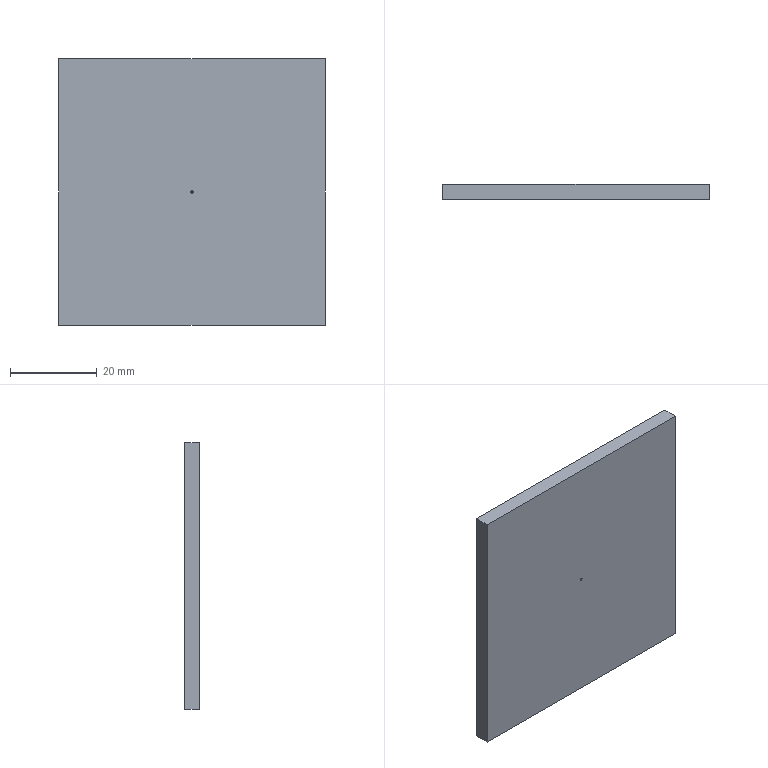Part | STEP file | 1 solid | 8 faces | box 61.25 x 3.43 x 61.25 mm | volume 12867 mm3 | plane 6 | cylinder 2 | commonest cylinder face diameters 0.49 x2
STEP:
#1=CARTESIAN_POINT('',(0.,0.,0.));
#2=DIRECTION('',(0.,0.,1.));
#3=DIRECTION('',(1.,0.,0.));
#4=AXIS2_PLACEMENT_3D('',#1,#2,#3);
#5=CARTESIAN_POINT('',(949.794,-61.739,161.762));
#6=VERTEX_POINT('',#5);
#7=CARTESIAN_POINT('',(950.284,-61.739,161.762));
#8=VERTEX_POINT('',#7);
#9=CARTESIAN_POINT('',(950.039,-61.739,161.762));
#10=DIRECTION('',(0.,-1.,0.));
#11=DIRECTION('',(-1.,0.,0.));
#12=AXIS2_PLACEMENT_3D('',#9,#10,#11);
#13=CIRCLE('',#12,0.245);
#14=CARTESIAN_POINT('',(950.039,-56.839,161.762));
#15=DIRECTION('',(0.,-1.,0.));
#16=DIRECTION('',(-1.,0.,0.));
#17=AXIS2_PLACEMENT_3D('',#14,#15,#16);
#18=CYLINDRICAL_SURFACE('',#17,0.245);
#19=CARTESIAN_POINT('',(0.,4.9));
#20=DIRECTION('',(1.,0.));
#21=VECTOR('',#20,1.);
#22=LINE('',#19,#21);
#23=(GEOMETRIC_REPRESENTATION_CONTEXT(2)PARAMETRIC_REPRESENTATION_CONTEXT()REPRESENTATION_CONTEXT('',''));
#24=DEFINITIONAL_REPRESENTATION('',(#22),#23);
#25=PCURVE('',#18,#24);
#26=CARTESIAN_POINT('',(980.664,-61.739,131.137));
#27=DIRECTION('',(0.,1.,0.));
#28=DIRECTION('',(0.,0.,-1.));
#29=AXIS2_PLACEMENT_3D('',#26,#27,#28);
#30=PLANE('',#29);
#31=CARTESIAN_POINT('',(-30.625,30.87));
#32=CARTESIAN_POINT('',(-30.201,30.87));
#33=CARTESIAN_POINT('',(-30.413,30.503));
#34=CARTESIAN_POINT('',(-30.625,30.135));
#35=CARTESIAN_POINT('',(-30.837,30.503));
#36=CARTESIAN_POINT('',(-31.049,30.87));
#37=CARTESIAN_POINT('',(-30.625,30.87));
#38=(BOUNDED_CURVE()B_SPLINE_CURVE(2,(#31,#32,#33,#34,#35,#36,#37),.UNSPECIFIED.,.T.,.F.)B_SPLINE_CURVE_WITH_KNOTS((1,2,2,2,2,1),(-2.094,0.,2.094,4.189,6.283,8.378),.UNSPECIFIED.)CURVE()GEOMETRIC_REPRESENTATION_ITEM()RATIONAL_B_SPLINE_CURVE((1.,0.5,1.,0.5,1.,0.5,1.))REPRESENTATION_ITEM(''));
#39=(GEOMETRIC_REPRESENTATION_CONTEXT(2)PARAMETRIC_REPRESENTATION_CONTEXT()REPRESENTATION_CONTEXT('',''));
#40=DEFINITIONAL_REPRESENTATION('',(#38),#39);
#41=PCURVE('',#30,#40);
#42=SURFACE_CURVE('',#13,(#25,#41),.PCURVE_S1.);
#43=EDGE_CURVE('',#6,#8,#42,.T.);
#44=ORIENTED_EDGE('',*,*,#43,.F.);
#45=CARTESIAN_POINT('',(949.794,-58.309,161.762));
#46=VERTEX_POINT('',#45);
#47=CARTESIAN_POINT('',(949.794,-56.839,161.762));
#48=DIRECTION('',(0.,-1.,0.));
#49=VECTOR('',#48,1.);
#50=LINE('',#47,#49);
#51=CARTESIAN_POINT('',(0.,0.));
#52=DIRECTION('',(0.,1.));
#53=VECTOR('',#52,1.);
#54=LINE('',#51,#53);
#55=(GEOMETRIC_REPRESENTATION_CONTEXT(2)PARAMETRIC_REPRESENTATION_CONTEXT()REPRESENTATION_CONTEXT('',''));
#56=DEFINITIONAL_REPRESENTATION('',(#54),#55);
#57=PCURVE('',#18,#56);
#58=CARTESIAN_POINT('',(950.039,-56.839,161.762));
#59=DIRECTION('',(0.,-1.,0.));
#60=DIRECTION('',(-1.,0.,0.));
#61=AXIS2_PLACEMENT_3D('',#58,#59,#60);
#62=CYLINDRICAL_SURFACE('',#61,0.245);
#63=CARTESIAN_POINT('',(6.283,0.));
#64=DIRECTION('',(0.,1.));
#65=VECTOR('',#64,1.);
#66=LINE('',#63,#65);
#67=(GEOMETRIC_REPRESENTATION_CONTEXT(2)PARAMETRIC_REPRESENTATION_CONTEXT()REPRESENTATION_CONTEXT('',''));
#68=DEFINITIONAL_REPRESENTATION('',(#66),#67);
#69=PCURVE('',#62,#68);
#70=SURFACE_CURVE('',#50,(#57,#69),.PCURVE_S1.);
#71=EDGE_CURVE('',#46,#6,#70,.T.);
#72=ORIENTED_EDGE('',*,*,#71,.F.);
#73=CARTESIAN_POINT('',(950.284,-58.309,161.762));
#74=VERTEX_POINT('',#73);
#75=CARTESIAN_POINT('',(950.039,-58.309,161.762));
#76=DIRECTION('',(0.,1.,0.));
#77=DIRECTION('',(1.,0.,0.));
#78=AXIS2_PLACEMENT_3D('',#75,#76,#77);
#79=CIRCLE('',#78,0.245);
#80=CARTESIAN_POINT('',(3.142,1.47));
#81=DIRECTION('',(-1.,0.));
#82=VECTOR('',#81,1.);
#83=LINE('',#80,#82);
#84=(GEOMETRIC_REPRESENTATION_CONTEXT(2)PARAMETRIC_REPRESENTATION_CONTEXT()REPRESENTATION_CONTEXT('',''));
#85=DEFINITIONAL_REPRESENTATION('',(#83),#84);
#86=PCURVE('',#18,#85);
#87=CARTESIAN_POINT('',(980.664,-58.309,131.137));
#88=DIRECTION('',(0.,1.,0.));
#89=DIRECTION('',(0.,0.,-1.));
#90=AXIS2_PLACEMENT_3D('',#87,#88,#89);
#91=PLANE('',#90);
#92=CARTESIAN_POINT('',(-30.625,30.625));
#93=DIRECTION('',(0.,-1.));
#94=AXIS2_PLACEMENT_2D('',#92,#93);
#95=CIRCLE('',#94,0.245);
#96=(GEOMETRIC_REPRESENTATION_CONTEXT(2)PARAMETRIC_REPRESENTATION_CONTEXT()REPRESENTATION_CONTEXT('',''));
#97=DEFINITIONAL_REPRESENTATION('',(#95),#96);
#98=PCURVE('',#91,#97);
#99=SURFACE_CURVE('',#79,(#86,#98),.PCURVE_S1.);
#100=EDGE_CURVE('',#74,#46,#99,.T.);
#101=ORIENTED_EDGE('',*,*,#100,.F.);
#102=CARTESIAN_POINT('',(950.284,-56.839,161.762));
#103=DIRECTION('',(0.,-1.,0.));
#104=VECTOR('',#103,1.);
#105=LINE('',#102,#104);
#106=CARTESIAN_POINT('',(3.142,0.));
#107=DIRECTION('',(0.,1.));
#108=VECTOR('',#107,1.);
#109=LINE('',#106,#108);
#110=(GEOMETRIC_REPRESENTATION_CONTEXT(2)PARAMETRIC_REPRESENTATION_CONTEXT()REPRESENTATION_CONTEXT('',''));
#111=DEFINITIONAL_REPRESENTATION('',(#109),#110);
#112=PCURVE('',#18,#111);
#113=CARTESIAN_POINT('',(3.142,0.));
#114=DIRECTION('',(0.,1.));
#115=VECTOR('',#114,1.);
#116=LINE('',#113,#115);
#117=(GEOMETRIC_REPRESENTATION_CONTEXT(2)PARAMETRIC_REPRESENTATION_CONTEXT()REPRESENTATION_CONTEXT('',''));
#118=DEFINITIONAL_REPRESENTATION('',(#116),#117);
#119=PCURVE('',#62,#118);
#120=SURFACE_CURVE('',#105,(#112,#119),.PCURVE_S1.);
#121=EDGE_CURVE('',#74,#8,#120,.T.);
#122=ORIENTED_EDGE('',*,*,#121,.T.);
#123=EDGE_LOOP('',(#44,#72,#101,#122));
#124=FACE_BOUND('',#123,.F.);
#125=ADVANCED_FACE('',(#124),#18,.F.);
#126=CARTESIAN_POINT('',(980.664,-61.739,192.387));
#127=VERTEX_POINT('',#126);
#128=CARTESIAN_POINT('',(919.414,-61.739,192.387));
#129=VERTEX_POINT('',#128);
#130=CARTESIAN_POINT('',(980.664,-61.739,192.387));
#131=DIRECTION('',(-1.,0.,0.));
#132=VECTOR('',#131,1.);
#133=LINE('',#130,#132);
#134=CARTESIAN_POINT('',(950.039,-58.309,192.387));
#135=DIRECTION('',(0.,0.,1.));
#136=DIRECTION('',(1.,0.,0.));
#137=AXIS2_PLACEMENT_3D('',#134,#135,#136);
#138=PLANE('',#137);
#139=CARTESIAN_POINT('',(30.625,-3.43));
#140=DIRECTION('',(-1.,0.));
#141=VECTOR('',#140,1.);
#142=LINE('',#139,#141);
#143=(GEOMETRIC_REPRESENTATION_CONTEXT(2)PARAMETRIC_REPRESENTATION_CONTEXT()REPRESENTATION_CONTEXT('',''));
#144=DEFINITIONAL_REPRESENTATION('',(#142),#143);
#145=PCURVE('',#138,#144);
#146=CARTESIAN_POINT('',(-61.25,0.));
#147=DIRECTION('',(0.,1.));
#148=VECTOR('',#147,1.);
#149=LINE('',#146,#148);
#150=(GEOMETRIC_REPRESENTATION_CONTEXT(2)PARAMETRIC_REPRESENTATION_CONTEXT()REPRESENTATION_CONTEXT('',''));
#151=DEFINITIONAL_REPRESENTATION('',(#149),#150);
#152=PCURVE('',#30,#151);
#153=SURFACE_CURVE('',#133,(#145,#152),.PCURVE_S1.);
#154=EDGE_CURVE('',#127,#129,#153,.T.);
#155=ORIENTED_EDGE('',*,*,#154,.F.);
#156=CARTESIAN_POINT('',(980.664,-58.309,192.387));
#157=VERTEX_POINT('',#156);
#158=CARTESIAN_POINT('',(980.664,-61.739,192.387));
#159=DIRECTION('',(0.,1.,0.));
#160=VECTOR('',#159,1.);
#161=LINE('',#158,#160);
#162=CARTESIAN_POINT('',(30.625,-3.43));
#163=DIRECTION('',(0.,1.));
#164=VECTOR('',#163,1.);
#165=LINE('',#162,#164);
#166=(GEOMETRIC_REPRESENTATION_CONTEXT(2)PARAMETRIC_REPRESENTATION_CONTEXT()REPRESENTATION_CONTEXT('',''));
#167=DEFINITIONAL_REPRESENTATION('',(#165),#166);
#168=PCURVE('',#138,#167);
#169=CARTESIAN_POINT('',(980.664,-61.739,131.137));
#170=DIRECTION('',(1.,0.,0.));
#171=DIRECTION('',(0.,0.,-1.));
#172=AXIS2_PLACEMENT_3D('',#169,#170,#171);
#173=PLANE('',#172);
#174=CARTESIAN_POINT('',(-61.25,0.));
#175=DIRECTION('',(0.,1.));
#176=VECTOR('',#175,1.);
#177=LINE('',#174,#176);
#178=(GEOMETRIC_REPRESENTATION_CONTEXT(2)PARAMETRIC_REPRESENTATION_CONTEXT()REPRESENTATION_CONTEXT('',''));
#179=DEFINITIONAL_REPRESENTATION('',(#177),#178);
#180=PCURVE('',#173,#179);
#181=SURFACE_CURVE('',#161,(#168,#180),.PCURVE_S1.);
#182=EDGE_CURVE('',#127,#157,#181,.T.);
#183=ORIENTED_EDGE('',*,*,#182,.T.);
#184=CARTESIAN_POINT('',(919.414,-58.309,192.387));
#185=VERTEX_POINT('',#184);
#186=CARTESIAN_POINT('',(980.664,-58.309,192.387));
#187=DIRECTION('',(-1.,0.,0.));
#188=VECTOR('',#187,1.);
#189=LINE('',#186,#188);
#190=CARTESIAN_POINT('',(30.625,0.));
#191=DIRECTION('',(-1.,0.));
#192=VECTOR('',#191,1.);
#193=LINE('',#190,#192);
#194=(GEOMETRIC_REPRESENTATION_CONTEXT(2)PARAMETRIC_REPRESENTATION_CONTEXT()REPRESENTATION_CONTEXT('',''));
#195=DEFINITIONAL_REPRESENTATION('',(#193),#194);
#196=PCURVE('',#138,#195);
#197=CARTESIAN_POINT('',(-61.25,0.));
#198=DIRECTION('',(0.,1.));
#199=VECTOR('',#198,1.);
#200=LINE('',#197,#199);
#201=(GEOMETRIC_REPRESENTATION_CONTEXT(2)PARAMETRIC_REPRESENTATION_CONTEXT()REPRESENTATION_CONTEXT('',''));
#202=DEFINITIONAL_REPRESENTATION('',(#200),#201);
#203=PCURVE('',#91,#202);
#204=SURFACE_CURVE('',#189,(#196,#203),.PCURVE_S1.);
#205=EDGE_CURVE('',#157,#185,#204,.T.);
#206=ORIENTED_EDGE('',*,*,#205,.T.);
#207=CARTESIAN_POINT('',(919.414,-58.309,192.387));
#208=DIRECTION('',(0.,-1.,0.));
#209=VECTOR('',#208,1.);
#210=LINE('',#207,#209);
#211=CARTESIAN_POINT('',(-30.625,0.));
#212=DIRECTION('',(0.,-1.));
#213=VECTOR('',#212,1.);
#214=LINE('',#211,#213);
#215=(GEOMETRIC_REPRESENTATION_CONTEXT(2)PARAMETRIC_REPRESENTATION_CONTEXT()REPRESENTATION_CONTEXT('',''));
#216=DEFINITIONAL_REPRESENTATION('',(#214),#215);
#217=PCURVE('',#138,#216);
#218=CARTESIAN_POINT('',(919.414,-58.309,131.137));
#219=DIRECTION('',(-1.,0.,0.));
#220=DIRECTION('',(0.,-1.,0.));
#221=AXIS2_PLACEMENT_3D('',#218,#219,#220);
#222=PLANE('',#221);
#223=CARTESIAN_POINT('',(0.,61.25));
#224=DIRECTION('',(1.,0.));
#225=VECTOR('',#224,1.);
#226=LINE('',#223,#225);
#227=(GEOMETRIC_REPRESENTATION_CONTEXT(2)PARAMETRIC_REPRESENTATION_CONTEXT()REPRESENTATION_CONTEXT('',''));
#228=DEFINITIONAL_REPRESENTATION('',(#226),#227);
#229=PCURVE('',#222,#228);
#230=SURFACE_CURVE('',#210,(#217,#229),.PCURVE_S1.);
#231=EDGE_CURVE('',#185,#129,#230,.T.);
#232=ORIENTED_EDGE('',*,*,#231,.T.);
#233=EDGE_LOOP('',(#155,#183,#206,#232));
#234=FACE_BOUND('',#233,.T.);
#235=ADVANCED_FACE('',(#234),#138,.T.);
#236=CARTESIAN_POINT('',(980.664,-61.739,131.137));
#237=VERTEX_POINT('',#236);
#238=CARTESIAN_POINT('',(919.414,-61.739,131.137));
#239=VERTEX_POINT('',#238);
#240=CARTESIAN_POINT('',(980.664,-61.739,131.137));
#241=DIRECTION('',(-1.,0.,0.));
#242=VECTOR('',#241,1.);
#243=LINE('',#240,#242);
#244=CARTESIAN_POINT('',(950.039,-58.309,131.137));
#245=DIRECTION('',(0.,0.,1.));
#246=DIRECTION('',(1.,0.,0.));
#247=AXIS2_PLACEMENT_3D('',#244,#245,#246);
#248=PLANE('',#247);
#249=CARTESIAN_POINT('',(30.625,-3.43));
#250=DIRECTION('',(-1.,0.));
#251=VECTOR('',#250,1.);
#252=LINE('',#249,#251);
#253=(GEOMETRIC_REPRESENTATION_CONTEXT(2)PARAMETRIC_REPRESENTATION_CONTEXT()REPRESENTATION_CONTEXT('',''));
#254=DEFINITIONAL_REPRESENTATION('',(#252),#253);
#255=PCURVE('',#248,#254);
#256=CARTESIAN_POINT('',(0.,0.));
#257=DIRECTION('',(0.,1.));
#258=VECTOR('',#257,1.);
#259=LINE('',#256,#258);
#260=(GEOMETRIC_REPRESENTATION_CONTEXT(2)PARAMETRIC_REPRESENTATION_CONTEXT()REPRESENTATION_CONTEXT('',''));
#261=DEFINITIONAL_REPRESENTATION('',(#259),#260);
#262=PCURVE('',#30,#261);
#263=SURFACE_CURVE('',#243,(#255,#262),.PCURVE_S1.);
#264=EDGE_CURVE('',#237,#239,#263,.T.);
#265=ORIENTED_EDGE('',*,*,#264,.T.);
#266=CARTESIAN_POINT('',(919.414,-58.309,131.137));
#267=VERTEX_POINT('',#266);
#268=CARTESIAN_POINT('',(919.414,-58.309,131.137));
#269=DIRECTION('',(0.,-1.,0.));
#270=VECTOR('',#269,1.);
#271=LINE('',#268,#270);
#272=CARTESIAN_POINT('',(-30.625,0.));
#273=DIRECTION('',(0.,-1.));
#274=VECTOR('',#273,1.);
#275=LINE('',#272,#274);
#276=(GEOMETRIC_REPRESENTATION_CONTEXT(2)PARAMETRIC_REPRESENTATION_CONTEXT()REPRESENTATION_CONTEXT('',''));
#277=DEFINITIONAL_REPRESENTATION('',(#275),#276);
#278=PCURVE('',#248,#277);
#279=CARTESIAN_POINT('',(0.,0.));
#280=DIRECTION('',(1.,0.));
#281=VECTOR('',#280,1.);
#282=LINE('',#279,#281);
#283=(GEOMETRIC_REPRESENTATION_CONTEXT(2)PARAMETRIC_REPRESENTATION_CONTEXT()REPRESENTATION_CONTEXT('',''));
#284=DEFINITIONAL_REPRESENTATION('',(#282),#283);
#285=PCURVE('',#222,#284);
#286=SURFACE_CURVE('',#271,(#278,#285),.PCURVE_S1.);
#287=EDGE_CURVE('',#267,#239,#286,.T.);
#288=ORIENTED_EDGE('',*,*,#287,.F.);
#289=CARTESIAN_POINT('',(980.664,-58.309,131.137));
#290=VERTEX_POINT('',#289);
#291=CARTESIAN_POINT('',(980.664,-58.309,131.137));
#292=DIRECTION('',(-1.,0.,0.));
#293=VECTOR('',#292,1.);
#294=LINE('',#291,#293);
#295=CARTESIAN_POINT('',(30.625,0.));
#296=DIRECTION('',(-1.,0.));
#297=VECTOR('',#296,1.);
#298=LINE('',#295,#297);
#299=(GEOMETRIC_REPRESENTATION_CONTEXT(2)PARAMETRIC_REPRESENTATION_CONTEXT()REPRESENTATION_CONTEXT('',''));
#300=DEFINITIONAL_REPRESENTATION('',(#298),#299);
#301=PCURVE('',#248,#300);
#302=CARTESIAN_POINT('',(0.,0.));
#303=DIRECTION('',(0.,1.));
#304=VECTOR('',#303,1.);
#305=LINE('',#302,#304);
#306=(GEOMETRIC_REPRESENTATION_CONTEXT(2)PARAMETRIC_REPRESENTATION_CONTEXT()REPRESENTATION_CONTEXT('',''));
#307=DEFINITIONAL_REPRESENTATION('',(#305),#306);
#308=PCURVE('',#91,#307);
#309=SURFACE_CURVE('',#294,(#301,#308),.PCURVE_S1.);
#310=EDGE_CURVE('',#290,#267,#309,.T.);
#311=ORIENTED_EDGE('',*,*,#310,.F.);
#312=CARTESIAN_POINT('',(980.664,-61.739,131.137));
#313=DIRECTION('',(0.,1.,0.));
#314=VECTOR('',#313,1.);
#315=LINE('',#312,#314);
#316=CARTESIAN_POINT('',(30.625,-3.43));
#317=DIRECTION('',(0.,1.));
#318=VECTOR('',#317,1.);
#319=LINE('',#316,#318);
#320=(GEOMETRIC_REPRESENTATION_CONTEXT(2)PARAMETRIC_REPRESENTATION_CONTEXT()REPRESENTATION_CONTEXT('',''));
#321=DEFINITIONAL_REPRESENTATION('',(#319),#320);
#322=PCURVE('',#248,#321);
#323=CARTESIAN_POINT('',(0.,0.));
#324=DIRECTION('',(0.,1.));
#325=VECTOR('',#324,1.);
#326=LINE('',#323,#325);
#327=(GEOMETRIC_REPRESENTATION_CONTEXT(2)PARAMETRIC_REPRESENTATION_CONTEXT()REPRESENTATION_CONTEXT('',''));
#328=DEFINITIONAL_REPRESENTATION('',(#326),#327);
#329=PCURVE('',#173,#328);
#330=SURFACE_CURVE('',#315,(#322,#329),.PCURVE_S1.);
#331=EDGE_CURVE('',#237,#290,#330,.T.);
#332=ORIENTED_EDGE('',*,*,#331,.F.);
#333=EDGE_LOOP('',(#265,#288,#311,#332));
#334=FACE_BOUND('',#333,.T.);
#335=ADVANCED_FACE('',(#334),#248,.F.);
#336=ORIENTED_EDGE('',*,*,#182,.F.);
#337=CARTESIAN_POINT('',(980.664,-61.739,131.137));
#338=DIRECTION('',(0.,0.,1.));
#339=VECTOR('',#338,1.);
#340=LINE('',#337,#339);
#341=CARTESIAN_POINT('',(0.,0.));
#342=DIRECTION('',(-1.,0.));
#343=VECTOR('',#342,1.);
#344=LINE('',#341,#343);
#345=(GEOMETRIC_REPRESENTATION_CONTEXT(2)PARAMETRIC_REPRESENTATION_CONTEXT()REPRESENTATION_CONTEXT('',''));
#346=DEFINITIONAL_REPRESENTATION('',(#344),#345);
#347=PCURVE('',#173,#346);
#348=CARTESIAN_POINT('',(0.,0.));
#349=DIRECTION('',(-1.,0.));
#350=VECTOR('',#349,1.);
#351=LINE('',#348,#350);
#352=(GEOMETRIC_REPRESENTATION_CONTEXT(2)PARAMETRIC_REPRESENTATION_CONTEXT()REPRESENTATION_CONTEXT('',''));
#353=DEFINITIONAL_REPRESENTATION('',(#351),#352);
#354=PCURVE('',#30,#353);
#355=SURFACE_CURVE('',#340,(#347,#354),.PCURVE_S1.);
#356=EDGE_CURVE('',#237,#127,#355,.T.);
#357=ORIENTED_EDGE('',*,*,#356,.F.);
#358=ORIENTED_EDGE('',*,*,#331,.T.);
#359=CARTESIAN_POINT('',(980.664,-58.309,131.137));
#360=DIRECTION('',(0.,0.,1.));
#361=VECTOR('',#360,1.);
#362=LINE('',#359,#361);
#363=CARTESIAN_POINT('',(0.,3.43));
#364=DIRECTION('',(-1.,0.));
#365=VECTOR('',#364,1.);
#366=LINE('',#363,#365);
#367=(GEOMETRIC_REPRESENTATION_CONTEXT(2)PARAMETRIC_REPRESENTATION_CONTEXT()REPRESENTATION_CONTEXT('',''));
#368=DEFINITIONAL_REPRESENTATION('',(#366),#367);
#369=PCURVE('',#173,#368);
#370=CARTESIAN_POINT('',(0.,0.));
#371=DIRECTION('',(-1.,0.));
#372=VECTOR('',#371,1.);
#373=LINE('',#370,#372);
#374=(GEOMETRIC_REPRESENTATION_CONTEXT(2)PARAMETRIC_REPRESENTATION_CONTEXT()REPRESENTATION_CONTEXT('',''));
#375=DEFINITIONAL_REPRESENTATION('',(#373),#374);
#376=PCURVE('',#91,#375);
#377=SURFACE_CURVE('',#362,(#369,#376),.PCURVE_S1.);
#378=EDGE_CURVE('',#290,#157,#377,.T.);
#379=ORIENTED_EDGE('',*,*,#378,.T.);
#380=EDGE_LOOP('',(#336,#357,#358,#379));
#381=FACE_BOUND('',#380,.T.);
#382=ADVANCED_FACE('',(#381),#173,.T.);
#383=CARTESIAN_POINT('',(950.039,-58.309,161.762));
#384=DIRECTION('',(0.,1.,0.));
#385=DIRECTION('',(1.,0.,0.));
#386=AXIS2_PLACEMENT_3D('',#383,#384,#385);
#387=CIRCLE('',#386,0.245);
#388=CARTESIAN_POINT('',(-30.625,30.625));
#389=DIRECTION('',(0.,-1.));
#390=AXIS2_PLACEMENT_2D('',#388,#389);
#391=CIRCLE('',#390,0.245);
#392=(GEOMETRIC_REPRESENTATION_CONTEXT(2)PARAMETRIC_REPRESENTATION_CONTEXT()REPRESENTATION_CONTEXT('',''));
#393=DEFINITIONAL_REPRESENTATION('',(#391),#392);
#394=PCURVE('',#91,#393);
#395=CARTESIAN_POINT('',(9.425,1.47));
#396=DIRECTION('',(-1.,0.));
#397=VECTOR('',#396,1.);
#398=LINE('',#395,#397);
#399=(GEOMETRIC_REPRESENTATION_CONTEXT(2)PARAMETRIC_REPRESENTATION_CONTEXT()REPRESENTATION_CONTEXT('',''));
#400=DEFINITIONAL_REPRESENTATION('',(#398),#399);
#401=PCURVE('',#62,#400);
#402=SURFACE_CURVE('',#387,(#394,#401),.PCURVE_S1.);
#403=EDGE_CURVE('',#46,#74,#402,.T.);
#404=ORIENTED_EDGE('',*,*,#403,.F.);
#405=ORIENTED_EDGE('',*,*,#100,.F.);
#406=EDGE_LOOP('',(#404,#405));
#407=FACE_BOUND('',#406,.T.);
#408=ORIENTED_EDGE('',*,*,#205,.F.);
#409=ORIENTED_EDGE('',*,*,#378,.F.);
#410=ORIENTED_EDGE('',*,*,#310,.T.);
#411=CARTESIAN_POINT('',(919.414,-58.309,131.137));
#412=DIRECTION('',(0.,0.,1.));
#413=VECTOR('',#412,1.);
#414=LINE('',#411,#413);
#415=CARTESIAN_POINT('',(0.,61.25));
#416=DIRECTION('',(-1.,0.));
#417=VECTOR('',#416,1.);
#418=LINE('',#415,#417);
#419=(GEOMETRIC_REPRESENTATION_CONTEXT(2)PARAMETRIC_REPRESENTATION_CONTEXT()REPRESENTATION_CONTEXT('',''));
#420=DEFINITIONAL_REPRESENTATION('',(#418),#419);
#421=PCURVE('',#91,#420);
#422=CARTESIAN_POINT('',(0.,0.));
#423=DIRECTION('',(0.,1.));
#424=VECTOR('',#423,1.);
#425=LINE('',#422,#424);
#426=(GEOMETRIC_REPRESENTATION_CONTEXT(2)PARAMETRIC_REPRESENTATION_CONTEXT()REPRESENTATION_CONTEXT('',''));
#427=DEFINITIONAL_REPRESENTATION('',(#425),#426);
#428=PCURVE('',#222,#427);
#429=SURFACE_CURVE('',#414,(#421,#428),.PCURVE_S1.);
#430=EDGE_CURVE('',#267,#185,#429,.T.);
#431=ORIENTED_EDGE('',*,*,#430,.T.);
#432=EDGE_LOOP('',(#408,#409,#410,#431));
#433=FACE_BOUND('',#432,.T.);
#434=ADVANCED_FACE('',(#407,#433),#91,.T.);
#435=ORIENTED_EDGE('',*,*,#231,.F.);
#436=ORIENTED_EDGE('',*,*,#430,.F.);
#437=ORIENTED_EDGE('',*,*,#287,.T.);
#438=CARTESIAN_POINT('',(919.414,-61.739,131.137));
#439=DIRECTION('',(0.,0.,1.));
#440=VECTOR('',#439,1.);
#441=LINE('',#438,#440);
#442=CARTESIAN_POINT('',(3.43,0.));
#443=DIRECTION('',(0.,1.));
#444=VECTOR('',#443,1.);
#445=LINE('',#442,#444);
#446=(GEOMETRIC_REPRESENTATION_CONTEXT(2)PARAMETRIC_REPRESENTATION_CONTEXT()REPRESENTATION_CONTEXT('',''));
#447=DEFINITIONAL_REPRESENTATION('',(#445),#446);
#448=PCURVE('',#222,#447);
#449=CARTESIAN_POINT('',(0.,61.25));
#450=DIRECTION('',(-1.,0.));
#451=VECTOR('',#450,1.);
#452=LINE('',#449,#451);
#453=(GEOMETRIC_REPRESENTATION_CONTEXT(2)PARAMETRIC_REPRESENTATION_CONTEXT()REPRESENTATION_CONTEXT('',''));
#454=DEFINITIONAL_REPRESENTATION('',(#452),#453);
#455=PCURVE('',#30,#454);
#456=SURFACE_CURVE('',#441,(#448,#455),.PCURVE_S1.);
#457=EDGE_CURVE('',#239,#129,#456,.T.);
#458=ORIENTED_EDGE('',*,*,#457,.T.);
#459=EDGE_LOOP('',(#435,#436,#437,#458));
#460=FACE_BOUND('',#459,.T.);
#461=ADVANCED_FACE('',(#460),#222,.T.);
#462=ORIENTED_EDGE('',*,*,#43,.F.);
#463=CARTESIAN_POINT('',(950.039,-61.739,161.762));
#464=DIRECTION('',(0.,-1.,0.));
#465=DIRECTION('',(-1.,0.,0.));
#466=AXIS2_PLACEMENT_3D('',#463,#464,#465);
#467=CIRCLE('',#466,0.245);
#468=CARTESIAN_POINT('',(-30.625,30.87));
#469=CARTESIAN_POINT('',(-30.201,30.87));
#470=CARTESIAN_POINT('',(-30.413,30.503));
#471=CARTESIAN_POINT('',(-30.625,30.135));
#472=CARTESIAN_POINT('',(-30.837,30.503));
#473=CARTESIAN_POINT('',(-31.049,30.87));
#474=CARTESIAN_POINT('',(-30.625,30.87));
#475=(BOUNDED_CURVE()B_SPLINE_CURVE(2,(#468,#469,#470,#471,#472,#473,#474),.UNSPECIFIED.,.T.,.F.)B_SPLINE_CURVE_WITH_KNOTS((1,2,2,2,2,1),(-2.094,0.,2.094,4.189,6.283,8.378),.UNSPECIFIED.)CURVE()GEOMETRIC_REPRESENTATION_ITEM()RATIONAL_B_SPLINE_CURVE((1.,0.5,1.,0.5,1.,0.5,1.))REPRESENTATION_ITEM(''));
#476=(GEOMETRIC_REPRESENTATION_CONTEXT(2)PARAMETRIC_REPRESENTATION_CONTEXT()REPRESENTATION_CONTEXT('',''));
#477=DEFINITIONAL_REPRESENTATION('',(#475),#476);
#478=PCURVE('',#30,#477);
#479=CARTESIAN_POINT('',(0.,4.9));
#480=DIRECTION('',(1.,0.));
#481=VECTOR('',#480,1.);
#482=LINE('',#479,#481);
#483=(GEOMETRIC_REPRESENTATION_CONTEXT(2)PARAMETRIC_REPRESENTATION_CONTEXT()REPRESENTATION_CONTEXT('',''));
#484=DEFINITIONAL_REPRESENTATION('',(#482),#483);
#485=PCURVE('',#62,#484);
#486=SURFACE_CURVE('',#467,(#478,#485),.PCURVE_S1.);
#487=EDGE_CURVE('',#8,#6,#486,.T.);
#488=ORIENTED_EDGE('',*,*,#487,.F.);
#489=EDGE_LOOP('',(#462,#488));
#490=FACE_BOUND('',#489,.T.);
#491=ORIENTED_EDGE('',*,*,#154,.T.);
#492=ORIENTED_EDGE('',*,*,#457,.F.);
#493=ORIENTED_EDGE('',*,*,#264,.F.);
#494=ORIENTED_EDGE('',*,*,#356,.T.);
#495=EDGE_LOOP('',(#491,#492,#493,#494));
#496=FACE_BOUND('',#495,.T.);
#497=ADVANCED_FACE('',(#490,#496),#30,.F.);
#498=ORIENTED_EDGE('',*,*,#71,.T.);
#499=ORIENTED_EDGE('',*,*,#487,.F.);
#500=ORIENTED_EDGE('',*,*,#121,.F.);
#501=ORIENTED_EDGE('',*,*,#403,.F.);
#502=EDGE_LOOP('',(#498,#499,#500,#501));
#503=FACE_BOUND('',#502,.F.);
#504=ADVANCED_FACE('',(#503),#62,.F.);
#505=CLOSED_SHELL('',(#125,#235,#335,#382,#434,#461,#497,#504));
#506=MANIFOLD_SOLID_BREP('',#505);
#507=(LENGTH_UNIT()NAMED_UNIT(*)SI_UNIT(.MILLI.,.METRE.));
#508=UNCERTAINTY_MEASURE_WITH_UNIT(LENGTH_MEASURE(0.0000001),#507,'','');
#509=(NAMED_UNIT(*)PLANE_ANGLE_UNIT()SI_UNIT($,.RADIAN.));
#510=(NAMED_UNIT(*)SI_UNIT($,.STERADIAN.)SOLID_ANGLE_UNIT());
#511=(GEOMETRIC_REPRESENTATION_CONTEXT(3)GLOBAL_UNCERTAINTY_ASSIGNED_CONTEXT((#508))GLOBAL_UNIT_ASSIGNED_CONTEXT((#507,#509,#510))REPRESENTATION_CONTEXT('',''));
#512=ADVANCED_BREP_SHAPE_REPRESENTATION('',(#4,#506),#511);